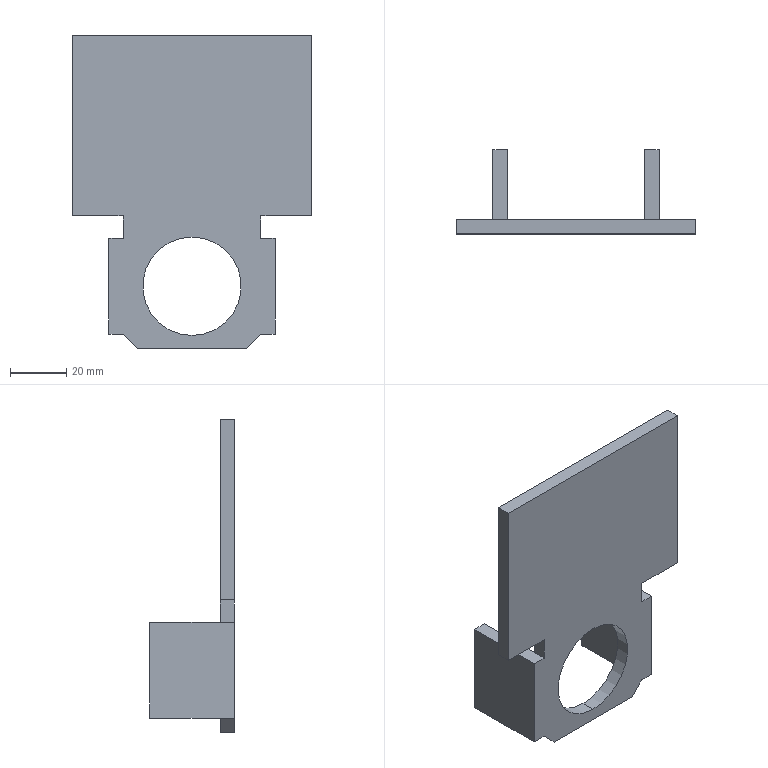Part | STEP file | Guide wheel mechanism revised.sldasm-Part-354 | 1 solid | 24 faces | box 85 x 30 x 111 mm | volume 43979 mm3 | plane 22 | cylinder 2 | commonest cylinder face diameters 35 x2
STEP:
#1=CARTESIAN_POINT('',(0.,0.,-17.5));
#2=VERTEX_POINT('',#1);
#3=CARTESIAN_POINT('',(0.,0.,17.5));
#4=VERTEX_POINT('',#3);
#5=CARTESIAN_POINT('',(0.,0.,0.));
#6=DIRECTION('',(0.,1.,0.));
#7=DIRECTION('',(0.,0.,1.));
#8=AXIS2_PLACEMENT_3D('',#5,#6,#7);
#9=CIRCLE('',#8,17.5);
#10=EDGE_CURVE('',#2,#4,#9,.T.);
#11=ORIENTED_EDGE('',*,*,#10,.F.);
#12=CARTESIAN_POINT('',(0.,5.,-17.5));
#13=VERTEX_POINT('',#12);
#14=CARTESIAN_POINT('',(0.,0.,-17.5));
#15=DIRECTION('',(0.,1.,0.));
#16=VECTOR('',#15,1000.);
#17=LINE('',#14,#16);
#18=EDGE_CURVE('',#2,#13,#17,.T.);
#19=ORIENTED_EDGE('',*,*,#18,.T.);
#20=CARTESIAN_POINT('',(0.,5.,17.5));
#21=VERTEX_POINT('',#20);
#22=CARTESIAN_POINT('',(0.,5.,0.));
#23=DIRECTION('',(0.,1.,0.));
#24=DIRECTION('',(0.,0.,1.));
#25=AXIS2_PLACEMENT_3D('',#22,#23,#24);
#26=CIRCLE('',#25,17.5);
#27=EDGE_CURVE('',#13,#21,#26,.T.);
#28=ORIENTED_EDGE('',*,*,#27,.T.);
#29=CARTESIAN_POINT('',(0.,0.,17.5));
#30=DIRECTION('',(0.,1.,0.));
#31=VECTOR('',#30,1000.);
#32=LINE('',#29,#31);
#33=EDGE_CURVE('',#4,#21,#32,.T.);
#34=ORIENTED_EDGE('',*,*,#33,.F.);
#35=EDGE_LOOP('',(#11,#19,#28,#34));
#36=FACE_OUTER_BOUND('',#35,.T.);
#37=CARTESIAN_POINT('',(0.,0.,0.));
#38=DIRECTION('',(0.,1.,0.));
#39=DIRECTION('',(0.,0.,1.));
#40=AXIS2_PLACEMENT_3D('',#37,#38,#39);
#41=CYLINDRICAL_SURFACE('',#40,17.5);
#42=ADVANCED_FACE('',(#36),#41,.F.);
#43=CARTESIAN_POINT('',(24.5,0.,17.));
#44=VERTEX_POINT('',#43);
#45=CARTESIAN_POINT('',(24.5,5.,17.));
#46=VERTEX_POINT('',#45);
#47=CARTESIAN_POINT('',(24.5,0.,17.));
#48=DIRECTION('',(0.,1.,0.));
#49=VECTOR('',#48,1000.);
#50=LINE('',#47,#49);
#51=EDGE_CURVE('',#44,#46,#50,.T.);
#52=ORIENTED_EDGE('',*,*,#51,.F.);
#53=CARTESIAN_POINT('',(29.5,0.,17.));
#54=VERTEX_POINT('',#53);
#55=CARTESIAN_POINT('',(-29.5,0.,17.));
#56=DIRECTION('',(1.,0.,0.));
#57=VECTOR('',#56,1000.);
#58=LINE('',#55,#57);
#59=EDGE_CURVE('',#44,#54,#58,.T.);
#60=ORIENTED_EDGE('',*,*,#59,.T.);
#61=CARTESIAN_POINT('',(29.5,30.,17.));
#62=VERTEX_POINT('',#61);
#63=CARTESIAN_POINT('',(29.5,0.,17.));
#64=DIRECTION('',(0.,1.,0.));
#65=VECTOR('',#64,1000.);
#66=LINE('',#63,#65);
#67=EDGE_CURVE('',#54,#62,#66,.T.);
#68=ORIENTED_EDGE('',*,*,#67,.T.);
#69=CARTESIAN_POINT('',(24.5,30.,17.));
#70=VERTEX_POINT('',#69);
#71=CARTESIAN_POINT('',(24.5,30.,17.));
#72=DIRECTION('',(1.,0.,0.));
#73=VECTOR('',#72,1000.);
#74=LINE('',#71,#73);
#75=EDGE_CURVE('',#70,#62,#74,.T.);
#76=ORIENTED_EDGE('',*,*,#75,.F.);
#77=CARTESIAN_POINT('',(24.5,0.,17.));
#78=DIRECTION('',(0.,1.,0.));
#79=VECTOR('',#78,1000.);
#80=LINE('',#77,#79);
#81=EDGE_CURVE('',#46,#70,#80,.T.);
#82=ORIENTED_EDGE('',*,*,#81,.F.);
#83=EDGE_LOOP('',(#52,#60,#68,#76,#82));
#84=FACE_OUTER_BOUND('',#83,.T.);
#85=CARTESIAN_POINT('',(0.,0.,17.));
#86=DIRECTION('',(0.,0.,-1.));
#87=DIRECTION('',(-1.,0.,0.));
#88=AXIS2_PLACEMENT_3D('',#85,#86,#87);
#89=PLANE('',#88);
#90=ADVANCED_FACE('',(#84),#89,.F.);
#91=CARTESIAN_POINT('',(24.5,0.,-17.));
#92=VERTEX_POINT('',#91);
#93=CARTESIAN_POINT('',(29.5,0.,-17.));
#94=VERTEX_POINT('',#93);
#95=CARTESIAN_POINT('',(-29.5,0.,-17.));
#96=DIRECTION('',(1.,0.,0.));
#97=VECTOR('',#96,1000.);
#98=LINE('',#95,#97);
#99=EDGE_CURVE('',#92,#94,#98,.T.);
#100=ORIENTED_EDGE('',*,*,#99,.F.);
#101=CARTESIAN_POINT('',(24.5,5.,-17.));
#102=VERTEX_POINT('',#101);
#103=CARTESIAN_POINT('',(24.5,-49.254,-17.));
#104=DIRECTION('',(0.,1.,0.));
#105=VECTOR('',#104,1000.);
#106=LINE('',#103,#105);
#107=EDGE_CURVE('',#92,#102,#106,.T.);
#108=ORIENTED_EDGE('',*,*,#107,.T.);
#109=CARTESIAN_POINT('',(24.5,30.,-17.));
#110=VERTEX_POINT('',#109);
#111=CARTESIAN_POINT('',(24.5,0.,-17.));
#112=DIRECTION('',(0.,1.,0.));
#113=VECTOR('',#112,1000.);
#114=LINE('',#111,#113);
#115=EDGE_CURVE('',#102,#110,#114,.T.);
#116=ORIENTED_EDGE('',*,*,#115,.T.);
#117=CARTESIAN_POINT('',(29.5,30.,-17.));
#118=VERTEX_POINT('',#117);
#119=CARTESIAN_POINT('',(24.5,30.,-17.));
#120=DIRECTION('',(1.,0.,0.));
#121=VECTOR('',#120,1000.);
#122=LINE('',#119,#121);
#123=EDGE_CURVE('',#110,#118,#122,.T.);
#124=ORIENTED_EDGE('',*,*,#123,.T.);
#125=CARTESIAN_POINT('',(29.5,0.,-17.));
#126=DIRECTION('',(0.,1.,0.));
#127=VECTOR('',#126,1000.);
#128=LINE('',#125,#127);
#129=EDGE_CURVE('',#94,#118,#128,.T.);
#130=ORIENTED_EDGE('',*,*,#129,.F.);
#131=EDGE_LOOP('',(#100,#108,#116,#124,#130));
#132=FACE_OUTER_BOUND('',#131,.T.);
#133=CARTESIAN_POINT('',(0.,0.,-17.));
#134=DIRECTION('',(0.,0.,-1.));
#135=DIRECTION('',(-1.,0.,0.));
#136=AXIS2_PLACEMENT_3D('',#133,#134,#135);
#137=PLANE('',#136);
#138=ADVANCED_FACE('',(#132),#137,.T.);
#139=ORIENTED_EDGE('',*,*,#129,.T.);
#140=CARTESIAN_POINT('',(29.5,30.,17.));
#141=DIRECTION('',(0.,0.,-1.));
#142=VECTOR('',#141,1000.);
#143=LINE('',#140,#142);
#144=EDGE_CURVE('',#62,#118,#143,.T.);
#145=ORIENTED_EDGE('',*,*,#144,.F.);
#146=ORIENTED_EDGE('',*,*,#67,.F.);
#147=CARTESIAN_POINT('',(29.5,0.,17.));
#148=DIRECTION('',(0.,0.,-1.));
#149=VECTOR('',#148,1000.);
#150=LINE('',#147,#149);
#151=EDGE_CURVE('',#54,#94,#150,.T.);
#152=ORIENTED_EDGE('',*,*,#151,.T.);
#153=EDGE_LOOP('',(#139,#145,#146,#152));
#154=FACE_OUTER_BOUND('',#153,.T.);
#155=CARTESIAN_POINT('',(29.5,0.,17.));
#156=DIRECTION('',(-1.,0.,0.));
#157=DIRECTION('',(0.,0.,1.));
#158=AXIS2_PLACEMENT_3D('',#155,#156,#157);
#159=PLANE('',#158);
#160=ADVANCED_FACE('',(#154),#159,.F.);
#161=ORIENTED_EDGE('',*,*,#123,.F.);
#162=CARTESIAN_POINT('',(24.5,30.,17.));
#163=DIRECTION('',(0.,0.,-1.));
#164=VECTOR('',#163,1000.);
#165=LINE('',#162,#164);
#166=EDGE_CURVE('',#70,#110,#165,.T.);
#167=ORIENTED_EDGE('',*,*,#166,.F.);
#168=ORIENTED_EDGE('',*,*,#75,.T.);
#169=ORIENTED_EDGE('',*,*,#144,.T.);
#170=EDGE_LOOP('',(#161,#167,#168,#169));
#171=FACE_OUTER_BOUND('',#170,.T.);
#172=CARTESIAN_POINT('',(24.5,30.,17.));
#173=DIRECTION('',(0.,1.,0.));
#174=DIRECTION('',(0.,0.,1.));
#175=AXIS2_PLACEMENT_3D('',#172,#173,#174);
#176=PLANE('',#175);
#177=ADVANCED_FACE('',(#171),#176,.T.);
#178=ORIENTED_EDGE('',*,*,#115,.F.);
#179=CARTESIAN_POINT('',(24.5,5.,17.));
#180=DIRECTION('',(0.,0.,-1.));
#181=VECTOR('',#180,1000.);
#182=LINE('',#179,#181);
#183=EDGE_CURVE('',#46,#102,#182,.T.);
#184=ORIENTED_EDGE('',*,*,#183,.F.);
#185=ORIENTED_EDGE('',*,*,#81,.T.);
#186=ORIENTED_EDGE('',*,*,#166,.T.);
#187=EDGE_LOOP('',(#178,#184,#185,#186));
#188=FACE_OUTER_BOUND('',#187,.T.);
#189=CARTESIAN_POINT('',(24.5,0.,17.));
#190=DIRECTION('',(-1.,0.,0.));
#191=DIRECTION('',(0.,0.,1.));
#192=AXIS2_PLACEMENT_3D('',#189,#190,#191);
#193=PLANE('',#192);
#194=ADVANCED_FACE('',(#188),#193,.T.);
#195=CARTESIAN_POINT('',(0.,5.,0.));
#196=DIRECTION('',(0.,1.,0.));
#197=DIRECTION('',(0.,0.,1.));
#198=AXIS2_PLACEMENT_3D('',#195,#196,#197);
#199=CIRCLE('',#198,17.5);
#200=EDGE_CURVE('',#21,#13,#199,.T.);
#201=ORIENTED_EDGE('',*,*,#200,.F.);
#202=ORIENTED_EDGE('',*,*,#27,.F.);
#203=EDGE_LOOP('',(#201,#202));
#204=FACE_BOUND('',#203,.T.);
#205=ORIENTED_EDGE('',*,*,#183,.T.);
#206=CARTESIAN_POINT('',(19.5,5.,-22.));
#207=VERTEX_POINT('',#206);
#208=CARTESIAN_POINT('',(14.5,5.,-27.));
#209=DIRECTION('',(-0.7071,0.,-0.7071));
#210=VECTOR('',#209,1000.);
#211=LINE('',#208,#210);
#212=EDGE_CURVE('',#102,#207,#211,.T.);
#213=ORIENTED_EDGE('',*,*,#212,.T.);
#214=CARTESIAN_POINT('',(-19.5,5.,-22.));
#215=VERTEX_POINT('',#214);
#216=CARTESIAN_POINT('',(-24.5,5.,-22.));
#217=DIRECTION('',(-1.,0.,0.));
#218=VECTOR('',#217,1000.);
#219=LINE('',#216,#218);
#220=EDGE_CURVE('',#207,#215,#219,.T.);
#221=ORIENTED_EDGE('',*,*,#220,.T.);
#222=CARTESIAN_POINT('',(-24.5,5.,-17.));
#223=VERTEX_POINT('',#222);
#224=CARTESIAN_POINT('',(-44.,5.,2.5));
#225=DIRECTION('',(-0.7071,0.,0.7071));
#226=VECTOR('',#225,1000.);
#227=LINE('',#224,#226);
#228=EDGE_CURVE('',#215,#223,#227,.T.);
#229=ORIENTED_EDGE('',*,*,#228,.T.);
#230=CARTESIAN_POINT('',(-24.5,5.,17.));
#231=VERTEX_POINT('',#230);
#232=CARTESIAN_POINT('',(-24.5,5.,17.));
#233=DIRECTION('',(0.,0.,-1.));
#234=VECTOR('',#233,1000.);
#235=LINE('',#232,#234);
#236=EDGE_CURVE('',#231,#223,#235,.T.);
#237=ORIENTED_EDGE('',*,*,#236,.F.);
#238=CARTESIAN_POINT('',(-24.5,5.,25.));
#239=VERTEX_POINT('',#238);
#240=CARTESIAN_POINT('',(-24.5,5.,25.));
#241=DIRECTION('',(0.,0.,-1.));
#242=VECTOR('',#241,1000.);
#243=LINE('',#240,#242);
#244=EDGE_CURVE('',#239,#231,#243,.T.);
#245=ORIENTED_EDGE('',*,*,#244,.F.);
#246=CARTESIAN_POINT('',(-42.5,5.,25.));
#247=VERTEX_POINT('',#246);
#248=CARTESIAN_POINT('',(-42.5,5.,25.));
#249=DIRECTION('',(1.,0.,0.));
#250=VECTOR('',#249,1000.);
#251=LINE('',#248,#250);
#252=EDGE_CURVE('',#247,#239,#251,.T.);
#253=ORIENTED_EDGE('',*,*,#252,.F.);
#254=CARTESIAN_POINT('',(-42.5,5.,89.));
#255=VERTEX_POINT('',#254);
#256=CARTESIAN_POINT('',(-42.5,5.,89.));
#257=DIRECTION('',(0.,0.,-1.));
#258=VECTOR('',#257,1000.);
#259=LINE('',#256,#258);
#260=EDGE_CURVE('',#255,#247,#259,.T.);
#261=ORIENTED_EDGE('',*,*,#260,.F.);
#262=CARTESIAN_POINT('',(42.5,5.,89.));
#263=VERTEX_POINT('',#262);
#264=CARTESIAN_POINT('',(42.5,5.,89.));
#265=DIRECTION('',(-1.,0.,0.));
#266=VECTOR('',#265,1000.);
#267=LINE('',#264,#266);
#268=EDGE_CURVE('',#263,#255,#267,.T.);
#269=ORIENTED_EDGE('',*,*,#268,.F.);
#270=CARTESIAN_POINT('',(42.5,5.,25.));
#271=VERTEX_POINT('',#270);
#272=CARTESIAN_POINT('',(42.5,5.,25.));
#273=DIRECTION('',(0.,0.,1.));
#274=VECTOR('',#273,1000.);
#275=LINE('',#272,#274);
#276=EDGE_CURVE('',#271,#263,#275,.T.);
#277=ORIENTED_EDGE('',*,*,#276,.F.);
#278=CARTESIAN_POINT('',(24.5,5.,25.));
#279=VERTEX_POINT('',#278);
#280=CARTESIAN_POINT('',(24.5,5.,25.));
#281=DIRECTION('',(1.,0.,0.));
#282=VECTOR('',#281,1000.);
#283=LINE('',#280,#282);
#284=EDGE_CURVE('',#279,#271,#283,.T.);
#285=ORIENTED_EDGE('',*,*,#284,.F.);
#286=CARTESIAN_POINT('',(24.5,5.,17.));
#287=DIRECTION('',(0.,0.,1.));
#288=VECTOR('',#287,1000.);
#289=LINE('',#286,#288);
#290=EDGE_CURVE('',#46,#279,#289,.T.);
#291=ORIENTED_EDGE('',*,*,#290,.F.);
#292=EDGE_LOOP('',(#205,#213,#221,#229,#237,#245,#253,#261,#269,#277,#285,#291));
#293=FACE_OUTER_BOUND('',#292,.T.);
#294=CARTESIAN_POINT('',(-29.5,5.,17.));
#295=DIRECTION('',(0.,1.,0.));
#296=DIRECTION('',(0.,0.,1.));
#297=AXIS2_PLACEMENT_3D('',#294,#295,#296);
#298=PLANE('',#297);
#299=ADVANCED_FACE('',(#204,#293),#298,.T.);
#300=CARTESIAN_POINT('',(-24.5,30.,-17.));
#301=VERTEX_POINT('',#300);
#302=CARTESIAN_POINT('',(-24.5,30.,-17.));
#303=DIRECTION('',(0.,-1.,0.));
#304=VECTOR('',#303,1000.);
#305=LINE('',#302,#304);
#306=EDGE_CURVE('',#301,#223,#305,.T.);
#307=ORIENTED_EDGE('',*,*,#306,.F.);
#308=CARTESIAN_POINT('',(-24.5,30.,17.));
#309=VERTEX_POINT('',#308);
#310=CARTESIAN_POINT('',(-24.5,30.,17.));
#311=DIRECTION('',(0.,0.,-1.));
#312=VECTOR('',#311,1000.);
#313=LINE('',#310,#312);
#314=EDGE_CURVE('',#309,#301,#313,.T.);
#315=ORIENTED_EDGE('',*,*,#314,.F.);
#316=CARTESIAN_POINT('',(-24.5,30.,17.));
#317=DIRECTION('',(0.,-1.,0.));
#318=VECTOR('',#317,1000.);
#319=LINE('',#316,#318);
#320=EDGE_CURVE('',#309,#231,#319,.T.);
#321=ORIENTED_EDGE('',*,*,#320,.T.);
#322=ORIENTED_EDGE('',*,*,#236,.T.);
#323=EDGE_LOOP('',(#307,#315,#321,#322));
#324=FACE_OUTER_BOUND('',#323,.T.);
#325=CARTESIAN_POINT('',(-24.5,30.,17.));
#326=DIRECTION('',(1.,0.,0.));
#327=DIRECTION('',(0.,0.,-1.));
#328=AXIS2_PLACEMENT_3D('',#325,#326,#327);
#329=PLANE('',#328);
#330=ADVANCED_FACE('',(#324),#329,.T.);
#331=CARTESIAN_POINT('',(-29.5,30.,-17.));
#332=VERTEX_POINT('',#331);
#333=CARTESIAN_POINT('',(-29.5,30.,-17.));
#334=DIRECTION('',(1.,0.,0.));
#335=VECTOR('',#334,1000.);
#336=LINE('',#333,#335);
#337=EDGE_CURVE('',#332,#301,#336,.T.);
#338=ORIENTED_EDGE('',*,*,#337,.F.);
#339=CARTESIAN_POINT('',(-29.5,30.,17.));
#340=VERTEX_POINT('',#339);
#341=CARTESIAN_POINT('',(-29.5,30.,17.));
#342=DIRECTION('',(0.,0.,-1.));
#343=VECTOR('',#342,1000.);
#344=LINE('',#341,#343);
#345=EDGE_CURVE('',#340,#332,#344,.T.);
#346=ORIENTED_EDGE('',*,*,#345,.F.);
#347=CARTESIAN_POINT('',(-29.5,30.,17.));
#348=DIRECTION('',(1.,0.,0.));
#349=VECTOR('',#348,1000.);
#350=LINE('',#347,#349);
#351=EDGE_CURVE('',#340,#309,#350,.T.);
#352=ORIENTED_EDGE('',*,*,#351,.T.);
#353=ORIENTED_EDGE('',*,*,#314,.T.);
#354=EDGE_LOOP('',(#338,#346,#352,#353));
#355=FACE_OUTER_BOUND('',#354,.T.);
#356=CARTESIAN_POINT('',(-29.5,30.,17.));
#357=DIRECTION('',(0.,1.,0.));
#358=DIRECTION('',(0.,0.,1.));
#359=AXIS2_PLACEMENT_3D('',#356,#357,#358);
#360=PLANE('',#359);
#361=ADVANCED_FACE('',(#355),#360,.T.);
#362=CARTESIAN_POINT('',(-29.5,0.,-17.));
#363=VERTEX_POINT('',#362);
#364=CARTESIAN_POINT('',(-29.5,30.,-17.));
#365=DIRECTION('',(0.,-1.,0.));
#366=VECTOR('',#365,1000.);
#367=LINE('',#364,#366);
#368=EDGE_CURVE('',#332,#363,#367,.T.);
#369=ORIENTED_EDGE('',*,*,#368,.T.);
#370=CARTESIAN_POINT('',(-29.5,0.,17.));
#371=VERTEX_POINT('',#370);
#372=CARTESIAN_POINT('',(-29.5,0.,17.));
#373=DIRECTION('',(0.,0.,-1.));
#374=VECTOR('',#373,1000.);
#375=LINE('',#372,#374);
#376=EDGE_CURVE('',#371,#363,#375,.T.);
#377=ORIENTED_EDGE('',*,*,#376,.F.);
#378=CARTESIAN_POINT('',(-29.5,30.,17.));
#379=DIRECTION('',(0.,-1.,0.));
#380=VECTOR('',#379,1000.);
#381=LINE('',#378,#380);
#382=EDGE_CURVE('',#340,#371,#381,.T.);
#383=ORIENTED_EDGE('',*,*,#382,.F.);
#384=ORIENTED_EDGE('',*,*,#345,.T.);
#385=EDGE_LOOP('',(#369,#377,#383,#384));
#386=FACE_OUTER_BOUND('',#385,.T.);
#387=CARTESIAN_POINT('',(-29.5,30.,17.));
#388=DIRECTION('',(1.,0.,0.));
#389=DIRECTION('',(0.,0.,-1.));
#390=AXIS2_PLACEMENT_3D('',#387,#388,#389);
#391=PLANE('',#390);
#392=ADVANCED_FACE('',(#386),#391,.F.);
#393=CARTESIAN_POINT('',(0.,0.,0.));
#394=DIRECTION('',(0.,1.,0.));
#395=DIRECTION('',(0.,0.,1.));
#396=AXIS2_PLACEMENT_3D('',#393,#394,#395);
#397=CIRCLE('',#396,17.5);
#398=EDGE_CURVE('',#4,#2,#397,.T.);
#399=ORIENTED_EDGE('',*,*,#398,.T.);
#400=ORIENTED_EDGE('',*,*,#10,.T.);
#401=EDGE_LOOP('',(#399,#400));
#402=FACE_BOUND('',#401,.T.);
#403=CARTESIAN_POINT('',(-19.5,0.,-22.));
#404=VERTEX_POINT('',#403);
#405=CARTESIAN_POINT('',(19.5,0.,-22.));
#406=VERTEX_POINT('',#405);
#407=CARTESIAN_POINT('',(-24.5,0.,-22.));
#408=DIRECTION('',(1.,0.,0.));
#409=VECTOR('',#408,1000.);
#410=LINE('',#407,#409);
#411=EDGE_CURVE('',#404,#406,#410,.T.);
#412=ORIENTED_EDGE('',*,*,#411,.T.);
#413=CARTESIAN_POINT('',(24.5,0.,-17.));
#414=DIRECTION('',(0.7071,0.,0.7071));
#415=VECTOR('',#414,1000.);
#416=LINE('',#413,#415);
#417=EDGE_CURVE('',#406,#92,#416,.T.);
#418=ORIENTED_EDGE('',*,*,#417,.T.);
#419=ORIENTED_EDGE('',*,*,#99,.T.);
#420=ORIENTED_EDGE('',*,*,#151,.F.);
#421=ORIENTED_EDGE('',*,*,#59,.F.);
#422=CARTESIAN_POINT('',(24.5,0.,25.));
#423=VERTEX_POINT('',#422);
#424=CARTESIAN_POINT('',(24.5,0.,17.));
#425=DIRECTION('',(0.,0.,1.));
#426=VECTOR('',#425,1000.);
#427=LINE('',#424,#426);
#428=EDGE_CURVE('',#44,#423,#427,.T.);
#429=ORIENTED_EDGE('',*,*,#428,.T.);
#430=CARTESIAN_POINT('',(42.5,0.,25.));
#431=VERTEX_POINT('',#430);
#432=CARTESIAN_POINT('',(24.5,0.,25.));
#433=DIRECTION('',(1.,0.,0.));
#434=VECTOR('',#433,1000.);
#435=LINE('',#432,#434);
#436=EDGE_CURVE('',#423,#431,#435,.T.);
#437=ORIENTED_EDGE('',*,*,#436,.T.);
#438=CARTESIAN_POINT('',(42.5,0.,89.));
#439=VERTEX_POINT('',#438);
#440=CARTESIAN_POINT('',(42.5,0.,25.));
#441=DIRECTION('',(0.,0.,1.));
#442=VECTOR('',#441,1000.);
#443=LINE('',#440,#442);
#444=EDGE_CURVE('',#431,#439,#443,.T.);
#445=ORIENTED_EDGE('',*,*,#444,.T.);
#446=CARTESIAN_POINT('',(-42.5,0.,89.));
#447=VERTEX_POINT('',#446);
#448=CARTESIAN_POINT('',(42.5,0.,89.));
#449=DIRECTION('',(-1.,0.,0.));
#450=VECTOR('',#449,1000.);
#451=LINE('',#448,#450);
#452=EDGE_CURVE('',#439,#447,#451,.T.);
#453=ORIENTED_EDGE('',*,*,#452,.T.);
#454=CARTESIAN_POINT('',(-42.5,0.,25.));
#455=VERTEX_POINT('',#454);
#456=CARTESIAN_POINT('',(-42.5,0.,89.));
#457=DIRECTION('',(0.,0.,-1.));
#458=VECTOR('',#457,1000.);
#459=LINE('',#456,#458);
#460=EDGE_CURVE('',#447,#455,#459,.T.);
#461=ORIENTED_EDGE('',*,*,#460,.T.);
#462=CARTESIAN_POINT('',(-24.5,0.,25.));
#463=VERTEX_POINT('',#462);
#464=CARTESIAN_POINT('',(-42.5,0.,25.));
#465=DIRECTION('',(1.,0.,0.));
#466=VECTOR('',#465,1000.);
#467=LINE('',#464,#466);
#468=EDGE_CURVE('',#455,#463,#467,.T.);
#469=ORIENTED_EDGE('',*,*,#468,.T.);
#470=CARTESIAN_POINT('',(-24.5,0.,17.));
#471=VERTEX_POINT('',#470);
#472=CARTESIAN_POINT('',(-24.5,0.,25.));
#473=DIRECTION('',(0.,0.,-1.));
#474=VECTOR('',#473,1000.);
#475=LINE('',#472,#474);
#476=EDGE_CURVE('',#463,#471,#475,.T.);
#477=ORIENTED_EDGE('',*,*,#476,.T.);
#478=CARTESIAN_POINT('',(-29.5,0.,17.));
#479=DIRECTION('',(1.,0.,0.));
#480=VECTOR('',#479,1000.);
#481=LINE('',#478,#480);
#482=EDGE_CURVE('',#371,#471,#481,.T.);
#483=ORIENTED_EDGE('',*,*,#482,.F.);
#484=ORIENTED_EDGE('',*,*,#376,.T.);
#485=CARTESIAN_POINT('',(-24.5,0.,-17.));
#486=VERTEX_POINT('',#485);
#487=CARTESIAN_POINT('',(-29.5,0.,-17.));
#488=DIRECTION('',(1.,0.,0.));
#489=VECTOR('',#488,1000.);
#490=LINE('',#487,#489);
#491=EDGE_CURVE('',#363,#486,#490,.T.);
#492=ORIENTED_EDGE('',*,*,#491,.T.);
#493=CARTESIAN_POINT('',(-19.5,0.,-22.));
#494=DIRECTION('',(0.7071,0.,-0.7071));
#495=VECTOR('',#494,1000.);
#496=LINE('',#493,#495);
#497=EDGE_CURVE('',#486,#404,#496,.T.);
#498=ORIENTED_EDGE('',*,*,#497,.T.);
#499=EDGE_LOOP('',(#412,#418,#419,#420,#421,#429,#437,#445,#453,#461,#469,#477,#483,#484,#492,#498));
#500=FACE_OUTER_BOUND('',#499,.T.);
#501=CARTESIAN_POINT('',(-29.5,0.,17.));
#502=DIRECTION('',(0.,1.,0.));
#503=DIRECTION('',(0.,0.,1.));
#504=AXIS2_PLACEMENT_3D('',#501,#502,#503);
#505=PLANE('',#504);
#506=ADVANCED_FACE('',(#402,#500),#505,.F.);
#507=ORIENTED_EDGE('',*,*,#482,.T.);
#508=CARTESIAN_POINT('',(-24.5,0.,17.));
#509=DIRECTION('',(0.,1.,0.));
#510=VECTOR('',#509,1000.);
#511=LINE('',#508,#510);
#512=EDGE_CURVE('',#471,#231,#511,.T.);
#513=ORIENTED_EDGE('',*,*,#512,.T.);
#514=ORIENTED_EDGE('',*,*,#320,.F.);
#515=ORIENTED_EDGE('',*,*,#351,.F.);
#516=ORIENTED_EDGE('',*,*,#382,.T.);
#517=EDGE_LOOP('',(#507,#513,#514,#515,#516));
#518=FACE_OUTER_BOUND('',#517,.T.);
#519=CARTESIAN_POINT('',(0.,0.,17.));
#520=DIRECTION('',(0.,0.,-1.));
#521=DIRECTION('',(-1.,0.,0.));
#522=AXIS2_PLACEMENT_3D('',#519,#520,#521);
#523=PLANE('',#522);
#524=ADVANCED_FACE('',(#518),#523,.F.);
#525=CARTESIAN_POINT('',(-24.5,-49.254,-17.));
#526=DIRECTION('',(0.,1.,0.));
#527=VECTOR('',#526,1000.);
#528=LINE('',#525,#527);
#529=EDGE_CURVE('',#486,#223,#528,.T.);
#530=ORIENTED_EDGE('',*,*,#529,.F.);
#531=ORIENTED_EDGE('',*,*,#491,.F.);
#532=ORIENTED_EDGE('',*,*,#368,.F.);
#533=ORIENTED_EDGE('',*,*,#337,.T.);
#534=ORIENTED_EDGE('',*,*,#306,.T.);
#535=EDGE_LOOP('',(#530,#531,#532,#533,#534));
#536=FACE_OUTER_BOUND('',#535,.T.);
#537=CARTESIAN_POINT('',(0.,0.,-17.));
#538=DIRECTION('',(0.,0.,-1.));
#539=DIRECTION('',(-1.,0.,0.));
#540=AXIS2_PLACEMENT_3D('',#537,#538,#539);
#541=PLANE('',#540);
#542=ADVANCED_FACE('',(#536),#541,.T.);
#543=ORIENTED_EDGE('',*,*,#220,.F.);
#544=CARTESIAN_POINT('',(19.5,-49.254,-22.));
#545=DIRECTION('',(0.,-1.,0.));
#546=VECTOR('',#545,1000.);
#547=LINE('',#544,#546);
#548=EDGE_CURVE('',#207,#406,#547,.T.);
#549=ORIENTED_EDGE('',*,*,#548,.T.);
#550=ORIENTED_EDGE('',*,*,#411,.F.);
#551=CARTESIAN_POINT('',(-19.5,-49.254,-22.));
#552=DIRECTION('',(0.,1.,0.));
#553=VECTOR('',#552,1000.);
#554=LINE('',#551,#553);
#555=EDGE_CURVE('',#404,#215,#554,.T.);
#556=ORIENTED_EDGE('',*,*,#555,.T.);
#557=EDGE_LOOP('',(#543,#549,#550,#556));
#558=FACE_OUTER_BOUND('',#557,.T.);
#559=CARTESIAN_POINT('',(-24.5,-49.254,-22.));
#560=DIRECTION('',(0.,0.,-1.));
#561=DIRECTION('',(-1.,0.,0.));
#562=AXIS2_PLACEMENT_3D('',#559,#560,#561);
#563=PLANE('',#562);
#564=ADVANCED_FACE('',(#558),#563,.T.);
#565=ORIENTED_EDGE('',*,*,#417,.F.);
#566=ORIENTED_EDGE('',*,*,#548,.F.);
#567=ORIENTED_EDGE('',*,*,#212,.F.);
#568=ORIENTED_EDGE('',*,*,#107,.F.);
#569=EDGE_LOOP('',(#565,#566,#567,#568));
#570=FACE_OUTER_BOUND('',#569,.T.);
#571=CARTESIAN_POINT('',(24.5,-49.254,-17.));
#572=DIRECTION('',(-0.7071,0.,0.7071));
#573=DIRECTION('',(0.,1.,0.));
#574=AXIS2_PLACEMENT_3D('',#571,#572,#573);
#575=PLANE('',#574);
#576=ADVANCED_FACE('',(#570),#575,.F.);
#577=ORIENTED_EDGE('',*,*,#497,.F.);
#578=ORIENTED_EDGE('',*,*,#529,.T.);
#579=ORIENTED_EDGE('',*,*,#228,.F.);
#580=ORIENTED_EDGE('',*,*,#555,.F.);
#581=EDGE_LOOP('',(#577,#578,#579,#580));
#582=FACE_OUTER_BOUND('',#581,.T.);
#583=CARTESIAN_POINT('',(-19.5,-49.254,-22.));
#584=DIRECTION('',(0.7071,0.,0.7071));
#585=DIRECTION('',(0.,1.,0.));
#586=AXIS2_PLACEMENT_3D('',#583,#584,#585);
#587=PLANE('',#586);
#588=ADVANCED_FACE('',(#582),#587,.F.);
#589=ORIENTED_EDGE('',*,*,#268,.T.);
#590=CARTESIAN_POINT('',(-42.5,0.,89.));
#591=DIRECTION('',(0.,1.,0.));
#592=VECTOR('',#591,1000.);
#593=LINE('',#590,#592);
#594=EDGE_CURVE('',#447,#255,#593,.T.);
#595=ORIENTED_EDGE('',*,*,#594,.F.);
#596=ORIENTED_EDGE('',*,*,#452,.F.);
#597=CARTESIAN_POINT('',(42.5,0.,89.));
#598=DIRECTION('',(0.,1.,0.));
#599=VECTOR('',#598,1000.);
#600=LINE('',#597,#599);
#601=EDGE_CURVE('',#439,#263,#600,.T.);
#602=ORIENTED_EDGE('',*,*,#601,.T.);
#603=EDGE_LOOP('',(#589,#595,#596,#602));
#604=FACE_OUTER_BOUND('',#603,.T.);
#605=CARTESIAN_POINT('',(42.5,0.,89.));
#606=DIRECTION('',(0.,0.,-1.));
#607=DIRECTION('',(-1.,0.,0.));
#608=AXIS2_PLACEMENT_3D('',#605,#606,#607);
#609=PLANE('',#608);
#610=ADVANCED_FACE('',(#604),#609,.F.);
#611=ORIENTED_EDGE('',*,*,#260,.T.);
#612=CARTESIAN_POINT('',(-42.5,0.,25.));
#613=DIRECTION('',(0.,1.,0.));
#614=VECTOR('',#613,1000.);
#615=LINE('',#612,#614);
#616=EDGE_CURVE('',#455,#247,#615,.T.);
#617=ORIENTED_EDGE('',*,*,#616,.F.);
#618=ORIENTED_EDGE('',*,*,#460,.F.);
#619=ORIENTED_EDGE('',*,*,#594,.T.);
#620=EDGE_LOOP('',(#611,#617,#618,#619));
#621=FACE_OUTER_BOUND('',#620,.T.);
#622=CARTESIAN_POINT('',(-42.5,0.,89.));
#623=DIRECTION('',(1.,0.,0.));
#624=DIRECTION('',(0.,0.,-1.));
#625=AXIS2_PLACEMENT_3D('',#622,#623,#624);
#626=PLANE('',#625);
#627=ADVANCED_FACE('',(#621),#626,.F.);
#628=ORIENTED_EDGE('',*,*,#252,.T.);
#629=CARTESIAN_POINT('',(-24.5,0.,25.));
#630=DIRECTION('',(0.,1.,0.));
#631=VECTOR('',#630,1000.);
#632=LINE('',#629,#631);
#633=EDGE_CURVE('',#463,#239,#632,.T.);
#634=ORIENTED_EDGE('',*,*,#633,.F.);
#635=ORIENTED_EDGE('',*,*,#468,.F.);
#636=ORIENTED_EDGE('',*,*,#616,.T.);
#637=EDGE_LOOP('',(#628,#634,#635,#636));
#638=FACE_OUTER_BOUND('',#637,.T.);
#639=CARTESIAN_POINT('',(-42.5,0.,25.));
#640=DIRECTION('',(0.,0.,1.));
#641=DIRECTION('',(1.,0.,0.));
#642=AXIS2_PLACEMENT_3D('',#639,#640,#641);
#643=PLANE('',#642);
#644=ADVANCED_FACE('',(#638),#643,.F.);
#645=ORIENTED_EDGE('',*,*,#244,.T.);
#646=ORIENTED_EDGE('',*,*,#512,.F.);
#647=ORIENTED_EDGE('',*,*,#476,.F.);
#648=ORIENTED_EDGE('',*,*,#633,.T.);
#649=EDGE_LOOP('',(#645,#646,#647,#648));
#650=FACE_OUTER_BOUND('',#649,.T.);
#651=CARTESIAN_POINT('',(-24.5,0.,25.));
#652=DIRECTION('',(1.,0.,0.));
#653=DIRECTION('',(0.,0.,-1.));
#654=AXIS2_PLACEMENT_3D('',#651,#652,#653);
#655=PLANE('',#654);
#656=ADVANCED_FACE('',(#650),#655,.F.);
#657=ORIENTED_EDGE('',*,*,#290,.T.);
#658=CARTESIAN_POINT('',(24.5,0.,25.));
#659=DIRECTION('',(0.,1.,0.));
#660=VECTOR('',#659,1000.);
#661=LINE('',#658,#660);
#662=EDGE_CURVE('',#423,#279,#661,.T.);
#663=ORIENTED_EDGE('',*,*,#662,.F.);
#664=ORIENTED_EDGE('',*,*,#428,.F.);
#665=ORIENTED_EDGE('',*,*,#51,.T.);
#666=EDGE_LOOP('',(#657,#663,#664,#665));
#667=FACE_OUTER_BOUND('',#666,.T.);
#668=CARTESIAN_POINT('',(24.5,0.,17.));
#669=DIRECTION('',(-1.,0.,0.));
#670=DIRECTION('',(0.,0.,1.));
#671=AXIS2_PLACEMENT_3D('',#668,#669,#670);
#672=PLANE('',#671);
#673=ADVANCED_FACE('',(#667),#672,.F.);
#674=ORIENTED_EDGE('',*,*,#284,.T.);
#675=CARTESIAN_POINT('',(42.5,0.,25.));
#676=DIRECTION('',(0.,1.,0.));
#677=VECTOR('',#676,1000.);
#678=LINE('',#675,#677);
#679=EDGE_CURVE('',#431,#271,#678,.T.);
#680=ORIENTED_EDGE('',*,*,#679,.F.);
#681=ORIENTED_EDGE('',*,*,#436,.F.);
#682=ORIENTED_EDGE('',*,*,#662,.T.);
#683=EDGE_LOOP('',(#674,#680,#681,#682));
#684=FACE_OUTER_BOUND('',#683,.T.);
#685=CARTESIAN_POINT('',(24.5,0.,25.));
#686=DIRECTION('',(0.,0.,1.));
#687=DIRECTION('',(1.,0.,0.));
#688=AXIS2_PLACEMENT_3D('',#685,#686,#687);
#689=PLANE('',#688);
#690=ADVANCED_FACE('',(#684),#689,.F.);
#691=ORIENTED_EDGE('',*,*,#276,.T.);
#692=ORIENTED_EDGE('',*,*,#601,.F.);
#693=ORIENTED_EDGE('',*,*,#444,.F.);
#694=ORIENTED_EDGE('',*,*,#679,.T.);
#695=EDGE_LOOP('',(#691,#692,#693,#694));
#696=FACE_OUTER_BOUND('',#695,.T.);
#697=CARTESIAN_POINT('',(42.5,0.,25.));
#698=DIRECTION('',(-1.,0.,0.));
#699=DIRECTION('',(0.,0.,1.));
#700=AXIS2_PLACEMENT_3D('',#697,#698,#699);
#701=PLANE('',#700);
#702=ADVANCED_FACE('',(#696),#701,.F.);
#703=ORIENTED_EDGE('',*,*,#18,.F.);
#704=ORIENTED_EDGE('',*,*,#398,.F.);
#705=ORIENTED_EDGE('',*,*,#33,.T.);
#706=ORIENTED_EDGE('',*,*,#200,.T.);
#707=EDGE_LOOP('',(#703,#704,#705,#706));
#708=FACE_OUTER_BOUND('',#707,.T.);
#709=CARTESIAN_POINT('',(0.,0.,0.));
#710=DIRECTION('',(0.,1.,0.));
#711=DIRECTION('',(0.,0.,1.));
#712=AXIS2_PLACEMENT_3D('',#709,#710,#711);
#713=CYLINDRICAL_SURFACE('',#712,17.5);
#714=ADVANCED_FACE('',(#708),#713,.F.);
#715=CLOSED_SHELL('',(#42,#90,#138,#160,#177,#194,#299,#330,#361,#392,#506,#524,#542,#564,#576,#588,#610,#627,#644,#656,#673,#690,#702,#714));
#716=MANIFOLD_SOLID_BREP('',#715);
#717=CARTESIAN_POINT('',(0.,0.,0.));
#718=DIRECTION('',(0.,0.,1.));
#719=DIRECTION('',(1.,0.,0.));
#720=AXIS2_PLACEMENT_3D('',#717,#718,#719);
#721=(LENGTH_UNIT()NAMED_UNIT(*)SI_UNIT(.MILLI.,.METRE.));
#722=UNCERTAINTY_MEASURE_WITH_UNIT(LENGTH_MEASURE(0.00001),#721,'','');
#723=(NAMED_UNIT(*)PLANE_ANGLE_UNIT()SI_UNIT($,.RADIAN.));
#724=(NAMED_UNIT(*)SI_UNIT($,.STERADIAN.)SOLID_ANGLE_UNIT());
#725=(GEOMETRIC_REPRESENTATION_CONTEXT(3)GLOBAL_UNCERTAINTY_ASSIGNED_CONTEXT((#722))GLOBAL_UNIT_ASSIGNED_CONTEXT((#721,#723,#724))REPRESENTATION_CONTEXT('',''));
#726=ADVANCED_BREP_SHAPE_REPRESENTATION('',(#716,#720),#725);